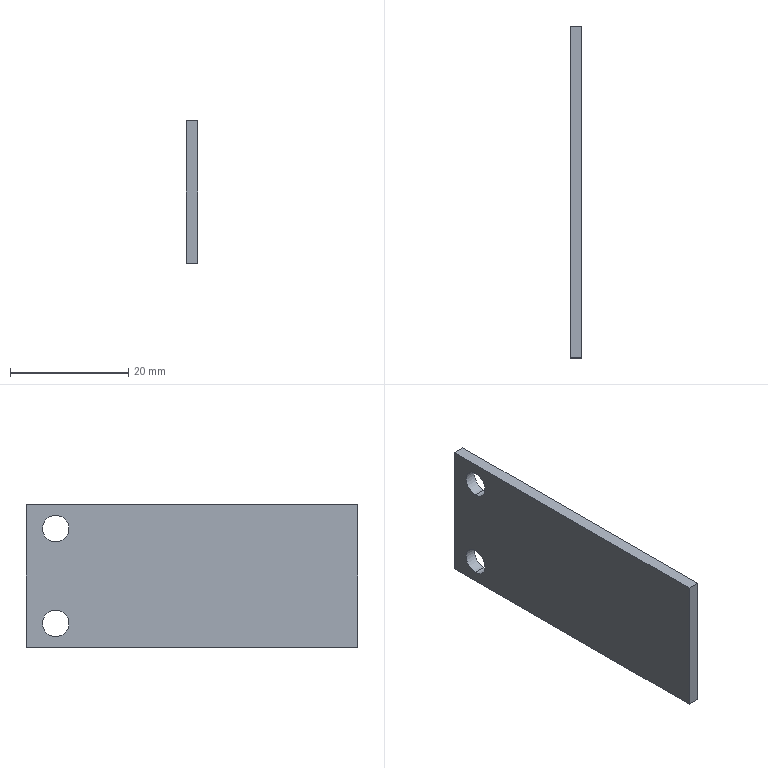Part | STEP file | PN_0043 sensor plate | 1 solid | 10 faces | box 2 x 56 x 24 mm | volume 2624 mm3 | plane 6 | cylinder 4 | commonest cylinder face diameters 4.5 x4
STEP:
#1=CARTESIAN_POINT('',(0.,0.,0.));
#2=DIRECTION('',(0.,0.,1.));
#3=DIRECTION('',(1.,0.,0.));
#4=AXIS2_PLACEMENT_3D('',#1,#2,#3);
#5=CARTESIAN_POINT('',(0.,51.,5.75));
#6=VERTEX_POINT('',#5);
#7=CARTESIAN_POINT('',(2.,51.,5.75));
#8=VERTEX_POINT('',#7);
#9=CARTESIAN_POINT('',(2.,51.,5.75));
#10=DIRECTION('',(1.,0.,0.));
#11=VECTOR('',#10,1.);
#12=LINE('',#9,#11);
#13=CARTESIAN_POINT('',(2.,51.,8.));
#14=DIRECTION('',(1.,0.,0.));
#15=DIRECTION('',(0.,0.,-1.));
#16=AXIS2_PLACEMENT_3D('',#13,#14,#15);
#17=CYLINDRICAL_SURFACE('',#16,2.25);
#18=CARTESIAN_POINT('',(6.283,0.));
#19=DIRECTION('',(0.,1.));
#20=VECTOR('',#19,1.);
#21=LINE('',#18,#20);
#22=(GEOMETRIC_REPRESENTATION_CONTEXT(2)PARAMETRIC_REPRESENTATION_CONTEXT()REPRESENTATION_CONTEXT('',''));
#23=DEFINITIONAL_REPRESENTATION('',(#21),#22);
#24=PCURVE('',#17,#23);
#25=CARTESIAN_POINT('',(2.,51.,8.));
#26=DIRECTION('',(1.,0.,0.));
#27=DIRECTION('',(0.,0.,-1.));
#28=AXIS2_PLACEMENT_3D('',#25,#26,#27);
#29=CYLINDRICAL_SURFACE('',#28,2.25);
#30=CARTESIAN_POINT('',(0.,0.));
#31=DIRECTION('',(0.,1.));
#32=VECTOR('',#31,1.);
#33=LINE('',#30,#32);
#34=(GEOMETRIC_REPRESENTATION_CONTEXT(2)PARAMETRIC_REPRESENTATION_CONTEXT()REPRESENTATION_CONTEXT('',''));
#35=DEFINITIONAL_REPRESENTATION('',(#33),#34);
#36=PCURVE('',#29,#35);
#37=SURFACE_CURVE('',#12,(#24,#36),.PCURVE_S1.);
#38=EDGE_CURVE('',#6,#8,#37,.T.);
#39=ORIENTED_EDGE('',*,*,#38,.T.);
#40=CARTESIAN_POINT('',(2.,51.,10.25));
#41=VERTEX_POINT('',#40);
#42=CARTESIAN_POINT('',(2.,51.,8.));
#43=DIRECTION('',(1.,0.,0.));
#44=DIRECTION('',(0.,0.,-1.));
#45=AXIS2_PLACEMENT_3D('',#42,#43,#44);
#46=CIRCLE('',#45,2.25);
#47=CARTESIAN_POINT('',(0.,0.));
#48=DIRECTION('',(1.,0.));
#49=VECTOR('',#48,1.);
#50=LINE('',#47,#49);
#51=(GEOMETRIC_REPRESENTATION_CONTEXT(2)PARAMETRIC_REPRESENTATION_CONTEXT()REPRESENTATION_CONTEXT('',''));
#52=DEFINITIONAL_REPRESENTATION('',(#50),#51);
#53=PCURVE('',#17,#52);
#54=CARTESIAN_POINT('',(2.,0.,0.));
#55=DIRECTION('',(-1.,0.,0.));
#56=DIRECTION('',(0.,0.,1.));
#57=AXIS2_PLACEMENT_3D('',#54,#55,#56);
#58=PLANE('',#57);
#59=CARTESIAN_POINT('',(5.75,51.));
#60=CARTESIAN_POINT('',(5.75,54.897));
#61=CARTESIAN_POINT('',(9.125,52.949));
#62=CARTESIAN_POINT('',(12.5,51.));
#63=CARTESIAN_POINT('',(9.125,49.051));
#64=CARTESIAN_POINT('',(5.75,47.103));
#65=CARTESIAN_POINT('',(5.75,51.));
#66=(BOUNDED_CURVE()B_SPLINE_CURVE(2,(#59,#60,#61,#62,#63,#64,#65),.UNSPECIFIED.,.T.,.F.)B_SPLINE_CURVE_WITH_KNOTS((1,2,2,2,2,1),(-2.094,0.,2.094,4.189,6.283,8.378),.UNSPECIFIED.)CURVE()GEOMETRIC_REPRESENTATION_ITEM()RATIONAL_B_SPLINE_CURVE((1.,0.5,1.,0.5,1.,0.5,1.))REPRESENTATION_ITEM(''));
#67=(GEOMETRIC_REPRESENTATION_CONTEXT(2)PARAMETRIC_REPRESENTATION_CONTEXT()REPRESENTATION_CONTEXT('',''));
#68=DEFINITIONAL_REPRESENTATION('',(#66),#67);
#69=PCURVE('',#58,#68);
#70=SURFACE_CURVE('',#46,(#53,#69),.PCURVE_S1.);
#71=EDGE_CURVE('',#41,#8,#70,.T.);
#72=ORIENTED_EDGE('',*,*,#71,.F.);
#73=CARTESIAN_POINT('',(0.,51.,10.25));
#74=VERTEX_POINT('',#73);
#75=CARTESIAN_POINT('',(2.,51.,10.25));
#76=DIRECTION('',(1.,0.,0.));
#77=VECTOR('',#76,1.);
#78=LINE('',#75,#77);
#79=CARTESIAN_POINT('',(3.142,0.));
#80=DIRECTION('',(0.,1.));
#81=VECTOR('',#80,1.);
#82=LINE('',#79,#81);
#83=(GEOMETRIC_REPRESENTATION_CONTEXT(2)PARAMETRIC_REPRESENTATION_CONTEXT()REPRESENTATION_CONTEXT('',''));
#84=DEFINITIONAL_REPRESENTATION('',(#82),#83);
#85=PCURVE('',#17,#84);
#86=CARTESIAN_POINT('',(3.142,0.));
#87=DIRECTION('',(0.,1.));
#88=VECTOR('',#87,1.);
#89=LINE('',#86,#88);
#90=(GEOMETRIC_REPRESENTATION_CONTEXT(2)PARAMETRIC_REPRESENTATION_CONTEXT()REPRESENTATION_CONTEXT('',''));
#91=DEFINITIONAL_REPRESENTATION('',(#89),#90);
#92=PCURVE('',#29,#91);
#93=SURFACE_CURVE('',#78,(#85,#92),.PCURVE_S1.);
#94=EDGE_CURVE('',#74,#41,#93,.T.);
#95=ORIENTED_EDGE('',*,*,#94,.F.);
#96=CARTESIAN_POINT('',(0.,51.,8.));
#97=DIRECTION('',(-1.,0.,0.));
#98=DIRECTION('',(0.,0.,1.));
#99=AXIS2_PLACEMENT_3D('',#96,#97,#98);
#100=CIRCLE('',#99,2.25);
#101=CARTESIAN_POINT('',(9.425,-2.));
#102=DIRECTION('',(-1.,0.));
#103=VECTOR('',#102,1.);
#104=LINE('',#101,#103);
#105=(GEOMETRIC_REPRESENTATION_CONTEXT(2)PARAMETRIC_REPRESENTATION_CONTEXT()REPRESENTATION_CONTEXT('',''));
#106=DEFINITIONAL_REPRESENTATION('',(#104),#105);
#107=PCURVE('',#17,#106);
#108=CARTESIAN_POINT('',(0.,0.,0.));
#109=DIRECTION('',(-1.,0.,0.));
#110=DIRECTION('',(0.,0.,1.));
#111=AXIS2_PLACEMENT_3D('',#108,#109,#110);
#112=PLANE('',#111);
#113=CARTESIAN_POINT('',(8.,51.));
#114=DIRECTION('',(1.,0.));
#115=AXIS2_PLACEMENT_2D('',#113,#114);
#116=CIRCLE('',#115,2.25);
#117=(GEOMETRIC_REPRESENTATION_CONTEXT(2)PARAMETRIC_REPRESENTATION_CONTEXT()REPRESENTATION_CONTEXT('',''));
#118=DEFINITIONAL_REPRESENTATION('',(#116),#117);
#119=PCURVE('',#112,#118);
#120=SURFACE_CURVE('',#100,(#107,#119),.PCURVE_S1.);
#121=EDGE_CURVE('',#6,#74,#120,.T.);
#122=ORIENTED_EDGE('',*,*,#121,.F.);
#123=EDGE_LOOP('',(#39,#72,#95,#122));
#124=FACE_BOUND('',#123,.F.);
#125=ADVANCED_FACE('',(#124),#17,.F.);
#126=CARTESIAN_POINT('',(0.,51.,-10.25));
#127=VERTEX_POINT('',#126);
#128=CARTESIAN_POINT('',(2.,51.,-10.25));
#129=VERTEX_POINT('',#128);
#130=CARTESIAN_POINT('',(2.,51.,-10.25));
#131=DIRECTION('',(1.,0.,0.));
#132=VECTOR('',#131,1.);
#133=LINE('',#130,#132);
#134=CARTESIAN_POINT('',(2.,51.,-8.));
#135=DIRECTION('',(1.,0.,0.));
#136=DIRECTION('',(0.,0.,-1.));
#137=AXIS2_PLACEMENT_3D('',#134,#135,#136);
#138=CYLINDRICAL_SURFACE('',#137,2.25);
#139=CARTESIAN_POINT('',(6.283,0.));
#140=DIRECTION('',(0.,1.));
#141=VECTOR('',#140,1.);
#142=LINE('',#139,#141);
#143=(GEOMETRIC_REPRESENTATION_CONTEXT(2)PARAMETRIC_REPRESENTATION_CONTEXT()REPRESENTATION_CONTEXT('',''));
#144=DEFINITIONAL_REPRESENTATION('',(#142),#143);
#145=PCURVE('',#138,#144);
#146=CARTESIAN_POINT('',(2.,51.,-8.));
#147=DIRECTION('',(1.,0.,0.));
#148=DIRECTION('',(0.,0.,-1.));
#149=AXIS2_PLACEMENT_3D('',#146,#147,#148);
#150=CYLINDRICAL_SURFACE('',#149,2.25);
#151=CARTESIAN_POINT('',(0.,0.));
#152=DIRECTION('',(0.,1.));
#153=VECTOR('',#152,1.);
#154=LINE('',#151,#153);
#155=(GEOMETRIC_REPRESENTATION_CONTEXT(2)PARAMETRIC_REPRESENTATION_CONTEXT()REPRESENTATION_CONTEXT('',''));
#156=DEFINITIONAL_REPRESENTATION('',(#154),#155);
#157=PCURVE('',#150,#156);
#158=SURFACE_CURVE('',#133,(#145,#157),.PCURVE_S1.);
#159=EDGE_CURVE('',#127,#129,#158,.T.);
#160=ORIENTED_EDGE('',*,*,#159,.T.);
#161=CARTESIAN_POINT('',(2.,51.,-5.75));
#162=VERTEX_POINT('',#161);
#163=CARTESIAN_POINT('',(2.,51.,-8.));
#164=DIRECTION('',(1.,0.,0.));
#165=DIRECTION('',(0.,0.,-1.));
#166=AXIS2_PLACEMENT_3D('',#163,#164,#165);
#167=CIRCLE('',#166,2.25);
#168=CARTESIAN_POINT('',(0.,0.));
#169=DIRECTION('',(1.,0.));
#170=VECTOR('',#169,1.);
#171=LINE('',#168,#170);
#172=(GEOMETRIC_REPRESENTATION_CONTEXT(2)PARAMETRIC_REPRESENTATION_CONTEXT()REPRESENTATION_CONTEXT('',''));
#173=DEFINITIONAL_REPRESENTATION('',(#171),#172);
#174=PCURVE('',#138,#173);
#175=CARTESIAN_POINT('',(-10.25,51.));
#176=CARTESIAN_POINT('',(-10.25,54.897));
#177=CARTESIAN_POINT('',(-6.875,52.949));
#178=CARTESIAN_POINT('',(-3.5,51.));
#179=CARTESIAN_POINT('',(-6.875,49.051));
#180=CARTESIAN_POINT('',(-10.25,47.103));
#181=CARTESIAN_POINT('',(-10.25,51.));
#182=(BOUNDED_CURVE()B_SPLINE_CURVE(2,(#175,#176,#177,#178,#179,#180,#181),.UNSPECIFIED.,.T.,.F.)B_SPLINE_CURVE_WITH_KNOTS((1,2,2,2,2,1),(-2.094,0.,2.094,4.189,6.283,8.378),.UNSPECIFIED.)CURVE()GEOMETRIC_REPRESENTATION_ITEM()RATIONAL_B_SPLINE_CURVE((1.,0.5,1.,0.5,1.,0.5,1.))REPRESENTATION_ITEM(''));
#183=(GEOMETRIC_REPRESENTATION_CONTEXT(2)PARAMETRIC_REPRESENTATION_CONTEXT()REPRESENTATION_CONTEXT('',''));
#184=DEFINITIONAL_REPRESENTATION('',(#182),#183);
#185=PCURVE('',#58,#184);
#186=SURFACE_CURVE('',#167,(#174,#185),.PCURVE_S1.);
#187=EDGE_CURVE('',#162,#129,#186,.T.);
#188=ORIENTED_EDGE('',*,*,#187,.F.);
#189=CARTESIAN_POINT('',(0.,51.,-5.75));
#190=VERTEX_POINT('',#189);
#191=CARTESIAN_POINT('',(2.,51.,-5.75));
#192=DIRECTION('',(1.,0.,0.));
#193=VECTOR('',#192,1.);
#194=LINE('',#191,#193);
#195=CARTESIAN_POINT('',(3.142,0.));
#196=DIRECTION('',(0.,1.));
#197=VECTOR('',#196,1.);
#198=LINE('',#195,#197);
#199=(GEOMETRIC_REPRESENTATION_CONTEXT(2)PARAMETRIC_REPRESENTATION_CONTEXT()REPRESENTATION_CONTEXT('',''));
#200=DEFINITIONAL_REPRESENTATION('',(#198),#199);
#201=PCURVE('',#138,#200);
#202=CARTESIAN_POINT('',(3.142,0.));
#203=DIRECTION('',(0.,1.));
#204=VECTOR('',#203,1.);
#205=LINE('',#202,#204);
#206=(GEOMETRIC_REPRESENTATION_CONTEXT(2)PARAMETRIC_REPRESENTATION_CONTEXT()REPRESENTATION_CONTEXT('',''));
#207=DEFINITIONAL_REPRESENTATION('',(#205),#206);
#208=PCURVE('',#150,#207);
#209=SURFACE_CURVE('',#194,(#201,#208),.PCURVE_S1.);
#210=EDGE_CURVE('',#190,#162,#209,.T.);
#211=ORIENTED_EDGE('',*,*,#210,.F.);
#212=CARTESIAN_POINT('',(0.,51.,-8.));
#213=DIRECTION('',(-1.,0.,0.));
#214=DIRECTION('',(0.,0.,1.));
#215=AXIS2_PLACEMENT_3D('',#212,#213,#214);
#216=CIRCLE('',#215,2.25);
#217=CARTESIAN_POINT('',(9.425,-2.));
#218=DIRECTION('',(-1.,0.));
#219=VECTOR('',#218,1.);
#220=LINE('',#217,#219);
#221=(GEOMETRIC_REPRESENTATION_CONTEXT(2)PARAMETRIC_REPRESENTATION_CONTEXT()REPRESENTATION_CONTEXT('',''));
#222=DEFINITIONAL_REPRESENTATION('',(#220),#221);
#223=PCURVE('',#138,#222);
#224=CARTESIAN_POINT('',(-8.,51.));
#225=DIRECTION('',(1.,0.));
#226=AXIS2_PLACEMENT_2D('',#224,#225);
#227=CIRCLE('',#226,2.25);
#228=(GEOMETRIC_REPRESENTATION_CONTEXT(2)PARAMETRIC_REPRESENTATION_CONTEXT()REPRESENTATION_CONTEXT('',''));
#229=DEFINITIONAL_REPRESENTATION('',(#227),#228);
#230=PCURVE('',#112,#229);
#231=SURFACE_CURVE('',#216,(#223,#230),.PCURVE_S1.);
#232=EDGE_CURVE('',#127,#190,#231,.T.);
#233=ORIENTED_EDGE('',*,*,#232,.F.);
#234=EDGE_LOOP('',(#160,#188,#211,#233));
#235=FACE_BOUND('',#234,.F.);
#236=ADVANCED_FACE('',(#235),#138,.F.);
#237=CARTESIAN_POINT('',(0.,56.,12.));
#238=VERTEX_POINT('',#237);
#239=CARTESIAN_POINT('',(0.,0.,12.));
#240=VERTEX_POINT('',#239);
#241=CARTESIAN_POINT('',(0.,0.,12.));
#242=DIRECTION('',(0.,-1.,0.));
#243=VECTOR('',#242,1.);
#244=LINE('',#241,#243);
#245=CARTESIAN_POINT('',(2.,0.,12.));
#246=DIRECTION('',(0.,0.,-1.));
#247=DIRECTION('',(-1.,0.,0.));
#248=AXIS2_PLACEMENT_3D('',#245,#246,#247);
#249=PLANE('',#248);
#250=CARTESIAN_POINT('',(2.,0.));
#251=DIRECTION('',(0.,-1.));
#252=VECTOR('',#251,1.);
#253=LINE('',#250,#252);
#254=(GEOMETRIC_REPRESENTATION_CONTEXT(2)PARAMETRIC_REPRESENTATION_CONTEXT()REPRESENTATION_CONTEXT('',''));
#255=DEFINITIONAL_REPRESENTATION('',(#253),#254);
#256=PCURVE('',#249,#255);
#257=CARTESIAN_POINT('',(12.,0.));
#258=DIRECTION('',(0.,-1.));
#259=VECTOR('',#258,1.);
#260=LINE('',#257,#259);
#261=(GEOMETRIC_REPRESENTATION_CONTEXT(2)PARAMETRIC_REPRESENTATION_CONTEXT()REPRESENTATION_CONTEXT('',''));
#262=DEFINITIONAL_REPRESENTATION('',(#260),#261);
#263=PCURVE('',#112,#262);
#264=SURFACE_CURVE('',#244,(#256,#263),.PCURVE_S1.);
#265=EDGE_CURVE('',#238,#240,#264,.T.);
#266=ORIENTED_EDGE('',*,*,#265,.T.);
#267=CARTESIAN_POINT('',(2.,0.,12.));
#268=VERTEX_POINT('',#267);
#269=CARTESIAN_POINT('',(2.,0.,12.));
#270=DIRECTION('',(-1.,0.,0.));
#271=VECTOR('',#270,1.);
#272=LINE('',#269,#271);
#273=CARTESIAN_POINT('',(0.,0.));
#274=DIRECTION('',(1.,0.));
#275=VECTOR('',#274,1.);
#276=LINE('',#273,#275);
#277=(GEOMETRIC_REPRESENTATION_CONTEXT(2)PARAMETRIC_REPRESENTATION_CONTEXT()REPRESENTATION_CONTEXT('',''));
#278=DEFINITIONAL_REPRESENTATION('',(#276),#277);
#279=PCURVE('',#249,#278);
#280=CARTESIAN_POINT('',(2.,0.,12.));
#281=DIRECTION('',(0.,1.,0.));
#282=DIRECTION('',(0.,0.,1.));
#283=AXIS2_PLACEMENT_3D('',#280,#281,#282);
#284=PLANE('',#283);
#285=CARTESIAN_POINT('',(0.,0.));
#286=DIRECTION('',(0.,-1.));
#287=VECTOR('',#286,1.);
#288=LINE('',#285,#287);
#289=(GEOMETRIC_REPRESENTATION_CONTEXT(2)PARAMETRIC_REPRESENTATION_CONTEXT()REPRESENTATION_CONTEXT('',''));
#290=DEFINITIONAL_REPRESENTATION('',(#288),#289);
#291=PCURVE('',#284,#290);
#292=SURFACE_CURVE('',#272,(#279,#291),.PCURVE_S1.);
#293=EDGE_CURVE('',#268,#240,#292,.T.);
#294=ORIENTED_EDGE('',*,*,#293,.F.);
#295=CARTESIAN_POINT('',(2.,56.,12.));
#296=VERTEX_POINT('',#295);
#297=CARTESIAN_POINT('',(2.,0.,12.));
#298=DIRECTION('',(0.,-1.,0.));
#299=VECTOR('',#298,1.);
#300=LINE('',#297,#299);
#301=CARTESIAN_POINT('',(0.,0.));
#302=DIRECTION('',(0.,-1.));
#303=VECTOR('',#302,1.);
#304=LINE('',#301,#303);
#305=(GEOMETRIC_REPRESENTATION_CONTEXT(2)PARAMETRIC_REPRESENTATION_CONTEXT()REPRESENTATION_CONTEXT('',''));
#306=DEFINITIONAL_REPRESENTATION('',(#304),#305);
#307=PCURVE('',#249,#306);
#308=CARTESIAN_POINT('',(12.,0.));
#309=DIRECTION('',(0.,-1.));
#310=VECTOR('',#309,1.);
#311=LINE('',#308,#310);
#312=(GEOMETRIC_REPRESENTATION_CONTEXT(2)PARAMETRIC_REPRESENTATION_CONTEXT()REPRESENTATION_CONTEXT('',''));
#313=DEFINITIONAL_REPRESENTATION('',(#311),#312);
#314=PCURVE('',#58,#313);
#315=SURFACE_CURVE('',#300,(#307,#314),.PCURVE_S1.);
#316=EDGE_CURVE('',#296,#268,#315,.T.);
#317=ORIENTED_EDGE('',*,*,#316,.F.);
#318=CARTESIAN_POINT('',(2.,56.,12.));
#319=DIRECTION('',(-1.,0.,0.));
#320=VECTOR('',#319,1.);
#321=LINE('',#318,#320);
#322=CARTESIAN_POINT('',(0.,56.));
#323=DIRECTION('',(1.,0.));
#324=VECTOR('',#323,1.);
#325=LINE('',#322,#324);
#326=(GEOMETRIC_REPRESENTATION_CONTEXT(2)PARAMETRIC_REPRESENTATION_CONTEXT()REPRESENTATION_CONTEXT('',''));
#327=DEFINITIONAL_REPRESENTATION('',(#325),#326);
#328=PCURVE('',#249,#327);
#329=CARTESIAN_POINT('',(2.,56.,12.));
#330=DIRECTION('',(0.,-1.,0.));
#331=DIRECTION('',(0.,0.,-1.));
#332=AXIS2_PLACEMENT_3D('',#329,#330,#331);
#333=PLANE('',#332);
#334=CARTESIAN_POINT('',(0.,0.));
#335=DIRECTION('',(0.,-1.));
#336=VECTOR('',#335,1.);
#337=LINE('',#334,#336);
#338=(GEOMETRIC_REPRESENTATION_CONTEXT(2)PARAMETRIC_REPRESENTATION_CONTEXT()REPRESENTATION_CONTEXT('',''));
#339=DEFINITIONAL_REPRESENTATION('',(#337),#338);
#340=PCURVE('',#333,#339);
#341=SURFACE_CURVE('',#321,(#328,#340),.PCURVE_S1.);
#342=EDGE_CURVE('',#296,#238,#341,.T.);
#343=ORIENTED_EDGE('',*,*,#342,.T.);
#344=EDGE_LOOP('',(#266,#294,#317,#343));
#345=FACE_BOUND('',#344,.T.);
#346=ADVANCED_FACE('',(#345),#249,.F.);
#347=CARTESIAN_POINT('',(0.,0.,-12.));
#348=VERTEX_POINT('',#347);
#349=CARTESIAN_POINT('',(0.,0.,12.));
#350=DIRECTION('',(0.,0.,-1.));
#351=VECTOR('',#350,1.);
#352=LINE('',#349,#351);
#353=CARTESIAN_POINT('',(0.,-2.));
#354=DIRECTION('',(-1.,0.));
#355=VECTOR('',#354,1.);
#356=LINE('',#353,#355);
#357=(GEOMETRIC_REPRESENTATION_CONTEXT(2)PARAMETRIC_REPRESENTATION_CONTEXT()REPRESENTATION_CONTEXT('',''));
#358=DEFINITIONAL_REPRESENTATION('',(#356),#357);
#359=PCURVE('',#284,#358);
#360=CARTESIAN_POINT('',(12.,0.));
#361=DIRECTION('',(-1.,0.));
#362=VECTOR('',#361,1.);
#363=LINE('',#360,#362);
#364=(GEOMETRIC_REPRESENTATION_CONTEXT(2)PARAMETRIC_REPRESENTATION_CONTEXT()REPRESENTATION_CONTEXT('',''));
#365=DEFINITIONAL_REPRESENTATION('',(#363),#364);
#366=PCURVE('',#112,#365);
#367=SURFACE_CURVE('',#352,(#359,#366),.PCURVE_S1.);
#368=EDGE_CURVE('',#240,#348,#367,.T.);
#369=ORIENTED_EDGE('',*,*,#368,.T.);
#370=CARTESIAN_POINT('',(2.,0.,-12.));
#371=VERTEX_POINT('',#370);
#372=CARTESIAN_POINT('',(2.,0.,-12.));
#373=DIRECTION('',(-1.,0.,0.));
#374=VECTOR('',#373,1.);
#375=LINE('',#372,#374);
#376=CARTESIAN_POINT('',(-24.,0.));
#377=DIRECTION('',(0.,-1.));
#378=VECTOR('',#377,1.);
#379=LINE('',#376,#378);
#380=(GEOMETRIC_REPRESENTATION_CONTEXT(2)PARAMETRIC_REPRESENTATION_CONTEXT()REPRESENTATION_CONTEXT('',''));
#381=DEFINITIONAL_REPRESENTATION('',(#379),#380);
#382=PCURVE('',#284,#381);
#383=CARTESIAN_POINT('',(2.,0.,-12.));
#384=DIRECTION('',(0.,0.,1.));
#385=DIRECTION('',(1.,0.,0.));
#386=AXIS2_PLACEMENT_3D('',#383,#384,#385);
#387=PLANE('',#386);
#388=CARTESIAN_POINT('',(0.,0.));
#389=DIRECTION('',(-1.,0.));
#390=VECTOR('',#389,1.);
#391=LINE('',#388,#390);
#392=(GEOMETRIC_REPRESENTATION_CONTEXT(2)PARAMETRIC_REPRESENTATION_CONTEXT()REPRESENTATION_CONTEXT('',''));
#393=DEFINITIONAL_REPRESENTATION('',(#391),#392);
#394=PCURVE('',#387,#393);
#395=SURFACE_CURVE('',#375,(#382,#394),.PCURVE_S1.);
#396=EDGE_CURVE('',#371,#348,#395,.T.);
#397=ORIENTED_EDGE('',*,*,#396,.F.);
#398=CARTESIAN_POINT('',(2.,0.,12.));
#399=DIRECTION('',(0.,0.,-1.));
#400=VECTOR('',#399,1.);
#401=LINE('',#398,#400);
#402=CARTESIAN_POINT('',(0.,0.));
#403=DIRECTION('',(-1.,0.));
#404=VECTOR('',#403,1.);
#405=LINE('',#402,#404);
#406=(GEOMETRIC_REPRESENTATION_CONTEXT(2)PARAMETRIC_REPRESENTATION_CONTEXT()REPRESENTATION_CONTEXT('',''));
#407=DEFINITIONAL_REPRESENTATION('',(#405),#406);
#408=PCURVE('',#284,#407);
#409=CARTESIAN_POINT('',(12.,0.));
#410=DIRECTION('',(-1.,0.));
#411=VECTOR('',#410,1.);
#412=LINE('',#409,#411);
#413=(GEOMETRIC_REPRESENTATION_CONTEXT(2)PARAMETRIC_REPRESENTATION_CONTEXT()REPRESENTATION_CONTEXT('',''));
#414=DEFINITIONAL_REPRESENTATION('',(#412),#413);
#415=PCURVE('',#58,#414);
#416=SURFACE_CURVE('',#401,(#408,#415),.PCURVE_S1.);
#417=EDGE_CURVE('',#268,#371,#416,.T.);
#418=ORIENTED_EDGE('',*,*,#417,.F.);
#419=ORIENTED_EDGE('',*,*,#293,.T.);
#420=EDGE_LOOP('',(#369,#397,#418,#419));
#421=FACE_BOUND('',#420,.T.);
#422=ADVANCED_FACE('',(#421),#284,.F.);
#423=CARTESIAN_POINT('',(0.,56.,-12.));
#424=VERTEX_POINT('',#423);
#425=CARTESIAN_POINT('',(0.,0.,-12.));
#426=DIRECTION('',(0.,1.,0.));
#427=VECTOR('',#426,1.);
#428=LINE('',#425,#427);
#429=CARTESIAN_POINT('',(-2.,0.));
#430=DIRECTION('',(0.,1.));
#431=VECTOR('',#430,1.);
#432=LINE('',#429,#431);
#433=(GEOMETRIC_REPRESENTATION_CONTEXT(2)PARAMETRIC_REPRESENTATION_CONTEXT()REPRESENTATION_CONTEXT('',''));
#434=DEFINITIONAL_REPRESENTATION('',(#432),#433);
#435=PCURVE('',#387,#434);
#436=CARTESIAN_POINT('',(-12.,0.));
#437=DIRECTION('',(0.,1.));
#438=VECTOR('',#437,1.);
#439=LINE('',#436,#438);
#440=(GEOMETRIC_REPRESENTATION_CONTEXT(2)PARAMETRIC_REPRESENTATION_CONTEXT()REPRESENTATION_CONTEXT('',''));
#441=DEFINITIONAL_REPRESENTATION('',(#439),#440);
#442=PCURVE('',#112,#441);
#443=SURFACE_CURVE('',#428,(#435,#442),.PCURVE_S1.);
#444=EDGE_CURVE('',#348,#424,#443,.T.);
#445=ORIENTED_EDGE('',*,*,#444,.T.);
#446=CARTESIAN_POINT('',(2.,56.,-12.));
#447=VERTEX_POINT('',#446);
#448=CARTESIAN_POINT('',(2.,56.,-12.));
#449=DIRECTION('',(-1.,0.,0.));
#450=VECTOR('',#449,1.);
#451=LINE('',#448,#450);
#452=CARTESIAN_POINT('',(0.,56.));
#453=DIRECTION('',(-1.,0.));
#454=VECTOR('',#453,1.);
#455=LINE('',#452,#454);
#456=(GEOMETRIC_REPRESENTATION_CONTEXT(2)PARAMETRIC_REPRESENTATION_CONTEXT()REPRESENTATION_CONTEXT('',''));
#457=DEFINITIONAL_REPRESENTATION('',(#455),#456);
#458=PCURVE('',#387,#457);
#459=CARTESIAN_POINT('',(24.,0.));
#460=DIRECTION('',(0.,-1.));
#461=VECTOR('',#460,1.);
#462=LINE('',#459,#461);
#463=(GEOMETRIC_REPRESENTATION_CONTEXT(2)PARAMETRIC_REPRESENTATION_CONTEXT()REPRESENTATION_CONTEXT('',''));
#464=DEFINITIONAL_REPRESENTATION('',(#462),#463);
#465=PCURVE('',#333,#464);
#466=SURFACE_CURVE('',#451,(#458,#465),.PCURVE_S1.);
#467=EDGE_CURVE('',#447,#424,#466,.T.);
#468=ORIENTED_EDGE('',*,*,#467,.F.);
#469=CARTESIAN_POINT('',(2.,0.,-12.));
#470=DIRECTION('',(0.,1.,0.));
#471=VECTOR('',#470,1.);
#472=LINE('',#469,#471);
#473=CARTESIAN_POINT('',(0.,0.));
#474=DIRECTION('',(0.,1.));
#475=VECTOR('',#474,1.);
#476=LINE('',#473,#475);
#477=(GEOMETRIC_REPRESENTATION_CONTEXT(2)PARAMETRIC_REPRESENTATION_CONTEXT()REPRESENTATION_CONTEXT('',''));
#478=DEFINITIONAL_REPRESENTATION('',(#476),#477);
#479=PCURVE('',#387,#478);
#480=CARTESIAN_POINT('',(-12.,0.));
#481=DIRECTION('',(0.,1.));
#482=VECTOR('',#481,1.);
#483=LINE('',#480,#482);
#484=(GEOMETRIC_REPRESENTATION_CONTEXT(2)PARAMETRIC_REPRESENTATION_CONTEXT()REPRESENTATION_CONTEXT('',''));
#485=DEFINITIONAL_REPRESENTATION('',(#483),#484);
#486=PCURVE('',#58,#485);
#487=SURFACE_CURVE('',#472,(#479,#486),.PCURVE_S1.);
#488=EDGE_CURVE('',#371,#447,#487,.T.);
#489=ORIENTED_EDGE('',*,*,#488,.F.);
#490=ORIENTED_EDGE('',*,*,#396,.T.);
#491=EDGE_LOOP('',(#445,#468,#489,#490));
#492=FACE_BOUND('',#491,.T.);
#493=ADVANCED_FACE('',(#492),#387,.F.);
#494=CARTESIAN_POINT('',(0.,56.,12.));
#495=DIRECTION('',(0.,0.,1.));
#496=VECTOR('',#495,1.);
#497=LINE('',#494,#496);
#498=CARTESIAN_POINT('',(0.,-2.));
#499=DIRECTION('',(-1.,0.));
#500=VECTOR('',#499,1.);
#501=LINE('',#498,#500);
#502=(GEOMETRIC_REPRESENTATION_CONTEXT(2)PARAMETRIC_REPRESENTATION_CONTEXT()REPRESENTATION_CONTEXT('',''));
#503=DEFINITIONAL_REPRESENTATION('',(#501),#502);
#504=PCURVE('',#333,#503);
#505=CARTESIAN_POINT('',(12.,56.));
#506=DIRECTION('',(1.,0.));
#507=VECTOR('',#506,1.);
#508=LINE('',#505,#507);
#509=(GEOMETRIC_REPRESENTATION_CONTEXT(2)PARAMETRIC_REPRESENTATION_CONTEXT()REPRESENTATION_CONTEXT('',''));
#510=DEFINITIONAL_REPRESENTATION('',(#508),#509);
#511=PCURVE('',#112,#510);
#512=SURFACE_CURVE('',#497,(#504,#511),.PCURVE_S1.);
#513=EDGE_CURVE('',#424,#238,#512,.T.);
#514=ORIENTED_EDGE('',*,*,#513,.T.);
#515=ORIENTED_EDGE('',*,*,#342,.F.);
#516=CARTESIAN_POINT('',(2.,56.,12.));
#517=DIRECTION('',(0.,0.,1.));
#518=VECTOR('',#517,1.);
#519=LINE('',#516,#518);
#520=CARTESIAN_POINT('',(0.,0.));
#521=DIRECTION('',(-1.,0.));
#522=VECTOR('',#521,1.);
#523=LINE('',#520,#522);
#524=(GEOMETRIC_REPRESENTATION_CONTEXT(2)PARAMETRIC_REPRESENTATION_CONTEXT()REPRESENTATION_CONTEXT('',''));
#525=DEFINITIONAL_REPRESENTATION('',(#523),#524);
#526=PCURVE('',#333,#525);
#527=CARTESIAN_POINT('',(12.,56.));
#528=DIRECTION('',(1.,0.));
#529=VECTOR('',#528,1.);
#530=LINE('',#527,#529);
#531=(GEOMETRIC_REPRESENTATION_CONTEXT(2)PARAMETRIC_REPRESENTATION_CONTEXT()REPRESENTATION_CONTEXT('',''));
#532=DEFINITIONAL_REPRESENTATION('',(#530),#531);
#533=PCURVE('',#58,#532);
#534=SURFACE_CURVE('',#519,(#526,#533),.PCURVE_S1.);
#535=EDGE_CURVE('',#447,#296,#534,.T.);
#536=ORIENTED_EDGE('',*,*,#535,.F.);
#537=ORIENTED_EDGE('',*,*,#467,.T.);
#538=EDGE_LOOP('',(#514,#515,#536,#537));
#539=FACE_BOUND('',#538,.T.);
#540=ADVANCED_FACE('',(#539),#333,.F.);
#541=CARTESIAN_POINT('',(2.,51.,8.));
#542=DIRECTION('',(1.,0.,0.));
#543=DIRECTION('',(0.,0.,-1.));
#544=AXIS2_PLACEMENT_3D('',#541,#542,#543);
#545=CIRCLE('',#544,2.25);
#546=CARTESIAN_POINT('',(5.75,51.));
#547=CARTESIAN_POINT('',(5.75,54.897));
#548=CARTESIAN_POINT('',(9.125,52.949));
#549=CARTESIAN_POINT('',(12.5,51.));
#550=CARTESIAN_POINT('',(9.125,49.051));
#551=CARTESIAN_POINT('',(5.75,47.103));
#552=CARTESIAN_POINT('',(5.75,51.));
#553=(BOUNDED_CURVE()B_SPLINE_CURVE(2,(#546,#547,#548,#549,#550,#551,#552),.UNSPECIFIED.,.T.,.F.)B_SPLINE_CURVE_WITH_KNOTS((1,2,2,2,2,1),(-2.094,0.,2.094,4.189,6.283,8.378),.UNSPECIFIED.)CURVE()GEOMETRIC_REPRESENTATION_ITEM()RATIONAL_B_SPLINE_CURVE((1.,0.5,1.,0.5,1.,0.5,1.))REPRESENTATION_ITEM(''));
#554=(GEOMETRIC_REPRESENTATION_CONTEXT(2)PARAMETRIC_REPRESENTATION_CONTEXT()REPRESENTATION_CONTEXT('',''));
#555=DEFINITIONAL_REPRESENTATION('',(#553),#554);
#556=PCURVE('',#58,#555);
#557=CARTESIAN_POINT('',(0.,0.));
#558=DIRECTION('',(1.,0.));
#559=VECTOR('',#558,1.);
#560=LINE('',#557,#559);
#561=(GEOMETRIC_REPRESENTATION_CONTEXT(2)PARAMETRIC_REPRESENTATION_CONTEXT()REPRESENTATION_CONTEXT('',''));
#562=DEFINITIONAL_REPRESENTATION('',(#560),#561);
#563=PCURVE('',#29,#562);
#564=SURFACE_CURVE('',#545,(#556,#563),.PCURVE_S1.);
#565=EDGE_CURVE('',#8,#41,#564,.T.);
#566=ORIENTED_EDGE('',*,*,#565,.F.);
#567=ORIENTED_EDGE('',*,*,#71,.F.);
#568=EDGE_LOOP('',(#566,#567));
#569=FACE_BOUND('',#568,.T.);
#570=CARTESIAN_POINT('',(2.,51.,-8.));
#571=DIRECTION('',(1.,0.,0.));
#572=DIRECTION('',(0.,0.,-1.));
#573=AXIS2_PLACEMENT_3D('',#570,#571,#572);
#574=CIRCLE('',#573,2.25);
#575=CARTESIAN_POINT('',(-10.25,51.));
#576=CARTESIAN_POINT('',(-10.25,54.897));
#577=CARTESIAN_POINT('',(-6.875,52.949));
#578=CARTESIAN_POINT('',(-3.5,51.));
#579=CARTESIAN_POINT('',(-6.875,49.051));
#580=CARTESIAN_POINT('',(-10.25,47.103));
#581=CARTESIAN_POINT('',(-10.25,51.));
#582=(BOUNDED_CURVE()B_SPLINE_CURVE(2,(#575,#576,#577,#578,#579,#580,#581),.UNSPECIFIED.,.T.,.F.)B_SPLINE_CURVE_WITH_KNOTS((1,2,2,2,2,1),(-2.094,0.,2.094,4.189,6.283,8.378),.UNSPECIFIED.)CURVE()GEOMETRIC_REPRESENTATION_ITEM()RATIONAL_B_SPLINE_CURVE((1.,0.5,1.,0.5,1.,0.5,1.))REPRESENTATION_ITEM(''));
#583=(GEOMETRIC_REPRESENTATION_CONTEXT(2)PARAMETRIC_REPRESENTATION_CONTEXT()REPRESENTATION_CONTEXT('',''));
#584=DEFINITIONAL_REPRESENTATION('',(#582),#583);
#585=PCURVE('',#58,#584);
#586=CARTESIAN_POINT('',(0.,0.));
#587=DIRECTION('',(1.,0.));
#588=VECTOR('',#587,1.);
#589=LINE('',#586,#588);
#590=(GEOMETRIC_REPRESENTATION_CONTEXT(2)PARAMETRIC_REPRESENTATION_CONTEXT()REPRESENTATION_CONTEXT('',''));
#591=DEFINITIONAL_REPRESENTATION('',(#589),#590);
#592=PCURVE('',#150,#591);
#593=SURFACE_CURVE('',#574,(#585,#592),.PCURVE_S1.);
#594=EDGE_CURVE('',#129,#162,#593,.T.);
#595=ORIENTED_EDGE('',*,*,#594,.F.);
#596=ORIENTED_EDGE('',*,*,#187,.F.);
#597=EDGE_LOOP('',(#595,#596));
#598=FACE_BOUND('',#597,.T.);
#599=ORIENTED_EDGE('',*,*,#316,.T.);
#600=ORIENTED_EDGE('',*,*,#417,.T.);
#601=ORIENTED_EDGE('',*,*,#488,.T.);
#602=ORIENTED_EDGE('',*,*,#535,.T.);
#603=EDGE_LOOP('',(#599,#600,#601,#602));
#604=FACE_BOUND('',#603,.T.);
#605=ADVANCED_FACE('',(#569,#598,#604),#58,.F.);
#606=ORIENTED_EDGE('',*,*,#121,.F.);
#607=CARTESIAN_POINT('',(0.,51.,8.));
#608=DIRECTION('',(-1.,0.,0.));
#609=DIRECTION('',(0.,0.,1.));
#610=AXIS2_PLACEMENT_3D('',#607,#608,#609);
#611=CIRCLE('',#610,2.25);
#612=CARTESIAN_POINT('',(8.,51.));
#613=DIRECTION('',(1.,0.));
#614=AXIS2_PLACEMENT_2D('',#612,#613);
#615=CIRCLE('',#614,2.25);
#616=(GEOMETRIC_REPRESENTATION_CONTEXT(2)PARAMETRIC_REPRESENTATION_CONTEXT()REPRESENTATION_CONTEXT('',''));
#617=DEFINITIONAL_REPRESENTATION('',(#615),#616);
#618=PCURVE('',#112,#617);
#619=CARTESIAN_POINT('',(3.142,-2.));
#620=DIRECTION('',(-1.,0.));
#621=VECTOR('',#620,1.);
#622=LINE('',#619,#621);
#623=(GEOMETRIC_REPRESENTATION_CONTEXT(2)PARAMETRIC_REPRESENTATION_CONTEXT()REPRESENTATION_CONTEXT('',''));
#624=DEFINITIONAL_REPRESENTATION('',(#622),#623);
#625=PCURVE('',#29,#624);
#626=SURFACE_CURVE('',#611,(#618,#625),.PCURVE_S1.);
#627=EDGE_CURVE('',#74,#6,#626,.T.);
#628=ORIENTED_EDGE('',*,*,#627,.F.);
#629=EDGE_LOOP('',(#606,#628));
#630=FACE_BOUND('',#629,.T.);
#631=ORIENTED_EDGE('',*,*,#232,.F.);
#632=CARTESIAN_POINT('',(0.,51.,-8.));
#633=DIRECTION('',(-1.,0.,0.));
#634=DIRECTION('',(0.,0.,1.));
#635=AXIS2_PLACEMENT_3D('',#632,#633,#634);
#636=CIRCLE('',#635,2.25);
#637=CARTESIAN_POINT('',(-8.,51.));
#638=DIRECTION('',(1.,0.));
#639=AXIS2_PLACEMENT_2D('',#637,#638);
#640=CIRCLE('',#639,2.25);
#641=(GEOMETRIC_REPRESENTATION_CONTEXT(2)PARAMETRIC_REPRESENTATION_CONTEXT()REPRESENTATION_CONTEXT('',''));
#642=DEFINITIONAL_REPRESENTATION('',(#640),#641);
#643=PCURVE('',#112,#642);
#644=CARTESIAN_POINT('',(3.142,-2.));
#645=DIRECTION('',(-1.,0.));
#646=VECTOR('',#645,1.);
#647=LINE('',#644,#646);
#648=(GEOMETRIC_REPRESENTATION_CONTEXT(2)PARAMETRIC_REPRESENTATION_CONTEXT()REPRESENTATION_CONTEXT('',''));
#649=DEFINITIONAL_REPRESENTATION('',(#647),#648);
#650=PCURVE('',#150,#649);
#651=SURFACE_CURVE('',#636,(#643,#650),.PCURVE_S1.);
#652=EDGE_CURVE('',#190,#127,#651,.T.);
#653=ORIENTED_EDGE('',*,*,#652,.F.);
#654=EDGE_LOOP('',(#631,#653));
#655=FACE_BOUND('',#654,.T.);
#656=ORIENTED_EDGE('',*,*,#265,.F.);
#657=ORIENTED_EDGE('',*,*,#513,.F.);
#658=ORIENTED_EDGE('',*,*,#444,.F.);
#659=ORIENTED_EDGE('',*,*,#368,.F.);
#660=EDGE_LOOP('',(#656,#657,#658,#659));
#661=FACE_BOUND('',#660,.T.);
#662=ADVANCED_FACE('',(#630,#655,#661),#112,.T.);
#663=ORIENTED_EDGE('',*,*,#594,.F.);
#664=ORIENTED_EDGE('',*,*,#159,.F.);
#665=ORIENTED_EDGE('',*,*,#652,.F.);
#666=ORIENTED_EDGE('',*,*,#210,.T.);
#667=EDGE_LOOP('',(#663,#664,#665,#666));
#668=FACE_BOUND('',#667,.F.);
#669=ADVANCED_FACE('',(#668),#150,.F.);
#670=ORIENTED_EDGE('',*,*,#565,.F.);
#671=ORIENTED_EDGE('',*,*,#38,.F.);
#672=ORIENTED_EDGE('',*,*,#627,.F.);
#673=ORIENTED_EDGE('',*,*,#94,.T.);
#674=EDGE_LOOP('',(#670,#671,#672,#673));
#675=FACE_BOUND('',#674,.F.);
#676=ADVANCED_FACE('',(#675),#29,.F.);
#677=CLOSED_SHELL('',(#125,#236,#346,#422,#493,#540,#605,#662,#669,#676));
#678=MANIFOLD_SOLID_BREP('',#677);
#679=(LENGTH_UNIT()NAMED_UNIT(*)SI_UNIT(.MILLI.,.METRE.));
#680=UNCERTAINTY_MEASURE_WITH_UNIT(LENGTH_MEASURE(0.0000001),#679,'','');
#681=(NAMED_UNIT(*)PLANE_ANGLE_UNIT()SI_UNIT($,.RADIAN.));
#682=(NAMED_UNIT(*)SI_UNIT($,.STERADIAN.)SOLID_ANGLE_UNIT());
#683=(GEOMETRIC_REPRESENTATION_CONTEXT(3)GLOBAL_UNCERTAINTY_ASSIGNED_CONTEXT((#680))GLOBAL_UNIT_ASSIGNED_CONTEXT((#679,#681,#682))REPRESENTATION_CONTEXT('',''));
#684=ADVANCED_BREP_SHAPE_REPRESENTATION('',(#4,#678),#683);